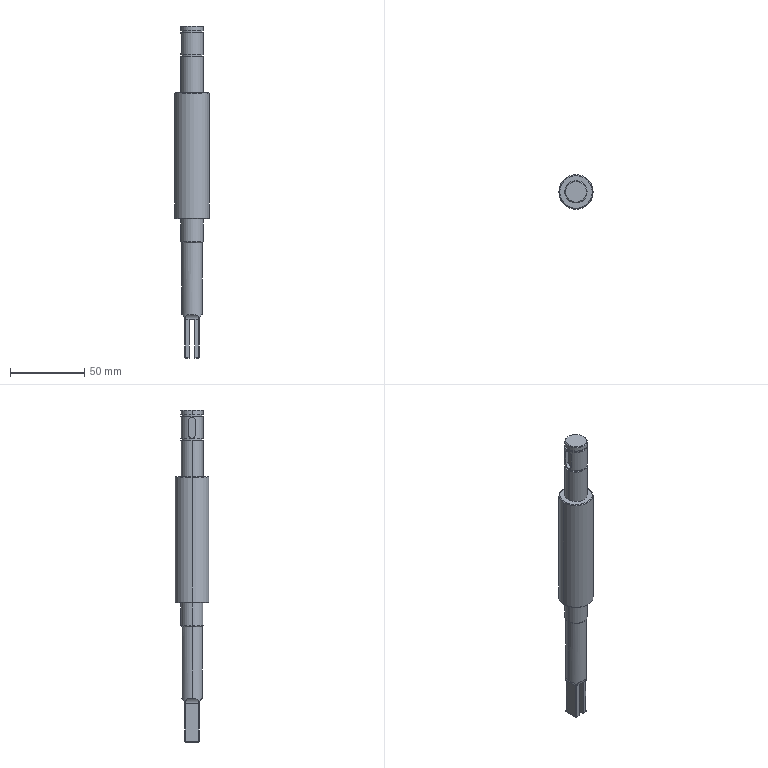Part | STEP file | Driven drive shaft SGN-5-06 | 1 solid | 74 faces | box 23 x 23 x 223.85 mm | volume 55141 mm3 | cylinder 35 | plane 21 | cone 10 | spline 4 | sphere 4 | commonest cylinder face diameters 1 x10 15 x8 8 x4 13.8 x4 5 x3 3.3 x2